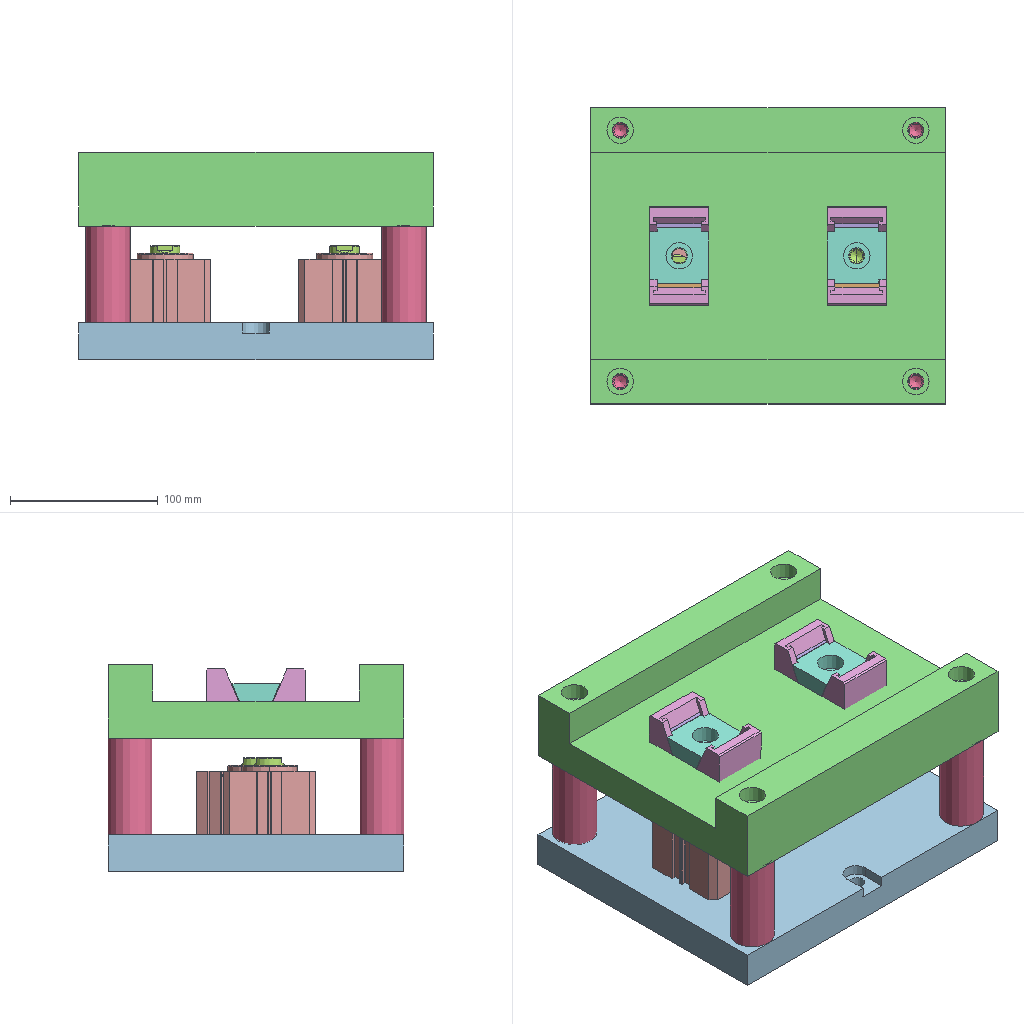Assembly | NX | 12 different items | 33 placed | box 240 x 200 x 140 mm
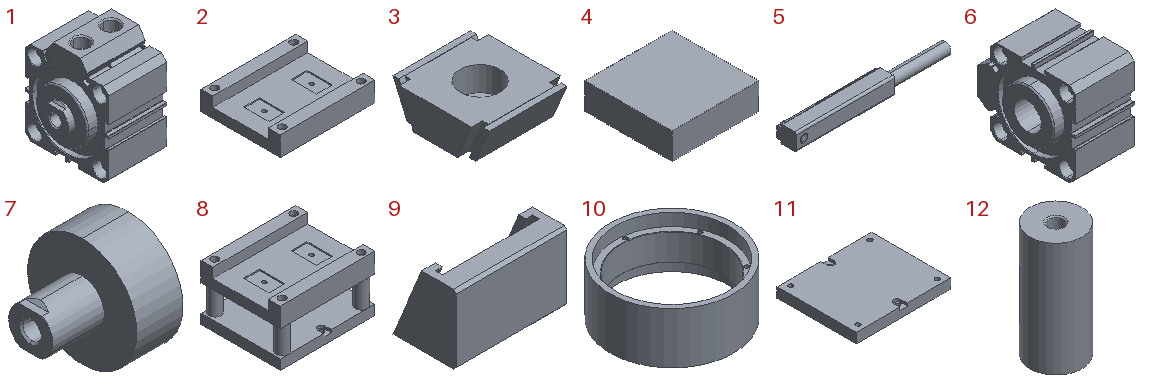Parts list (item | quantity | parent item | size | volume | features):
1 | x2 | - | 52 x 62 x 71.5 mm | 290253 mm3 | features BREP 3
2 | x1 | - | 240 x 200 x 50 mm | 1515162 mm3 | features EXTRUDE 6, DATUM_CSYS 4, SKETCH 3
3 | x2 | - | 40 x 43.514 x 15 mm | 17811 mm3 | features DATUM_CSYS 5, SKETCH 4, EXTRUDE 3, CBORE_HOLE 1, HOLE PACKAGE 1
4 | x1 | - | 82 x 82 x 25 mm | 237764 mm3 | features EXTRUDE 16, DATUM_CSYS 8, SKETCH 7, CHAMFER 5, BLEND 3, EXTRACT_STRING 2, DATUM_PLANE 1, HOLE PACKAGE 1, INTERSECTION_CURVES 1, Instance Feature 1, Mirror Feature 1, SIMPLE HOLE 1, SYMBOLIC_THREAD 1
5 | x8 | in 1 | 40.5 x 5.8 x 4.4 mm | 628.81 mm3 | features BREP 1
6 | x4 | in 1 | 47 x 71.5 x 62 mm | 97197 mm3 | features BREP 1
7 | x4 | in 1 | 44.5 x 49.5 x 49.5 mm | 46672 mm3 | features BREP 1
8 | x1 | - | 240 x 200 x 141 mm | 2862487 mm3 | features EXTRUDE 12, DATUM_CSYS 9, SKETCH 6, HOLE PACKAGE 2, SIMPLE HOLE 2, SYMBOLIC_THREAD 2, DATUM_PLANE 1
9 | x4 | - | 40 x 22.855 x 25 mm | 13567 mm3 | features DATUM_CSYS 3, EXTRUDE 2, SKETCH 2
10 | x1 | - | 120 x 120 x 50 mm | 139903 mm3 | features Instance Feature 6, SYMBOLIC_THREAD 6, DATUM_CSYS 5, IDENTICAL INSTANCE OUTPUT 5, EXTRUDE 4, SKETCH 4, EXTRACT_FACE 2, EXTRACT_STRING 2, CHAMFER 1, DATUM_PLANE 1, HOLE PACKAGE 1, MASTER SNAPSHOT BODY 1, Mirror Feature 1, Pattern Feature 1, SIMPLE HOLE 1
11 | x1 | - | 240 x 200 x 25 mm | 1174329 mm3 | features EXTRUDE 5, DATUM_CSYS 3, SKETCH 2, DATUM_PLANE 1
12 | x4 | - | 30 x 30 x 66 mm | 43249 mm3 | features DATUM_CSYS 2, HOLE PACKAGE 2, SIMPLE HOLE 2, SYMBOLIC_THREAD 2, EXTRUDE 1, SKETCH 1
Mates (type | each side: item.copy, entity, surface, feature):
Concentric | 12.1 arc | 11.1 edge
Concentric | 12.1 | 11.1 edge | 3 times
Touch | 2.1 face plane Extrude(2) | 12.1 face plane Extrude(2)
AlignLock | 2.1 edge | 12.1 edge
Touch | 3.1 face plane Extrude(2) | 2.1 face plane Extrude(12) | 2 times
AlignLock | 3.1 edge | 2.1 edge
AlignLock | 3.1 face cylinder Ø11 Counterbored Hole(8) | 2.1 face cylinder Extrude(11)
Touch | 9.1 face plane Extrude(8) | 3.1 face plane Extrude(6) | 8 times
AlignLock | 9.1 edge | 3.1 edge | 4 times
Touch | 6.1 face plane Body(1) | 11.1 face plane Extrude(2) | 2 times